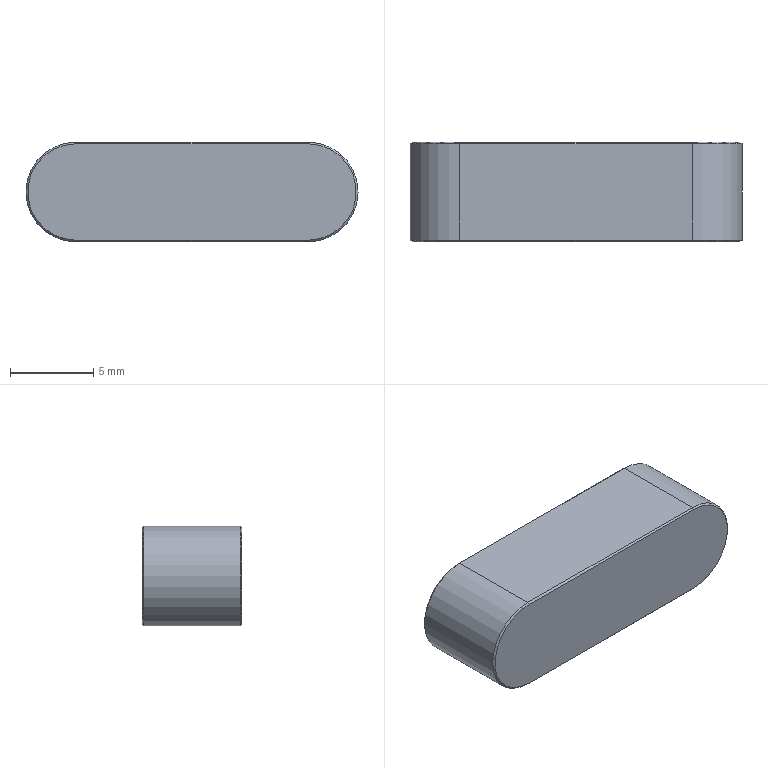Part | STEP file | Type A key 6x6 20L | 1 solid | 14 faces | box 20 x 6 x 6 mm | volume 673.18 mm3 | plane 8 | cone 4 | cylinder 2 | commonest cylinder face diameters 6 x2
STEP:
#1=CARTESIAN_POINT('',(0.,0.,0.));
#2=DIRECTION('',(0.,0.,1.));
#3=DIRECTION('',(1.,0.,0.));
#4=AXIS2_PLACEMENT_3D('',#1,#2,#3);
#5=CARTESIAN_POINT('',(-7.,2.9,-3.));
#6=VERTEX_POINT('',#5);
#7=CARTESIAN_POINT('',(-7.,-2.9,-3.));
#8=VERTEX_POINT('',#7);
#9=CARTESIAN_POINT('',(-7.,3.,-3.));
#10=DIRECTION('',(0.,-1.,0.));
#11=VECTOR('',#10,1.);
#12=LINE('',#9,#11);
#13=CARTESIAN_POINT('',(-7.,3.,0.));
#14=DIRECTION('',(0.,-1.,0.));
#15=DIRECTION('',(0.,0.,-1.));
#16=AXIS2_PLACEMENT_3D('',#13,#14,#15);
#17=CYLINDRICAL_SURFACE('',#16,3.);
#18=CARTESIAN_POINT('',(6.283,0.));
#19=DIRECTION('',(0.,1.));
#20=VECTOR('',#19,1.);
#21=LINE('',#18,#20);
#22=(GEOMETRIC_REPRESENTATION_CONTEXT(2)PARAMETRIC_REPRESENTATION_CONTEXT()REPRESENTATION_CONTEXT('',''));
#23=DEFINITIONAL_REPRESENTATION('',(#21),#22);
#24=PCURVE('',#17,#23);
#25=CARTESIAN_POINT('',(-7.,3.,-3.));
#26=DIRECTION('',(0.,0.,1.));
#27=DIRECTION('',(1.,0.,0.));
#28=AXIS2_PLACEMENT_3D('',#25,#26,#27);
#29=PLANE('',#28);
#30=CARTESIAN_POINT('',(0.,0.));
#31=DIRECTION('',(0.,-1.));
#32=VECTOR('',#31,1.);
#33=LINE('',#30,#32);
#34=(GEOMETRIC_REPRESENTATION_CONTEXT(2)PARAMETRIC_REPRESENTATION_CONTEXT()REPRESENTATION_CONTEXT('',''));
#35=DEFINITIONAL_REPRESENTATION('',(#33),#34);
#36=PCURVE('',#29,#35);
#37=SURFACE_CURVE('',#12,(#24,#36),.PCURVE_S1.);
#38=EDGE_CURVE('',#6,#8,#37,.T.);
#39=ORIENTED_EDGE('',*,*,#38,.T.);
#40=CARTESIAN_POINT('',(-7.,-2.9,3.));
#41=VERTEX_POINT('',#40);
#42=CARTESIAN_POINT('',(-7.,-2.9,0.));
#43=DIRECTION('',(0.,1.,0.));
#44=DIRECTION('',(0.,0.,1.));
#45=AXIS2_PLACEMENT_3D('',#42,#43,#44);
#46=CIRCLE('',#45,3.);
#47=CARTESIAN_POINT('',(9.425,5.9));
#48=DIRECTION('',(-1.,0.));
#49=VECTOR('',#48,1.);
#50=LINE('',#47,#49);
#51=(GEOMETRIC_REPRESENTATION_CONTEXT(2)PARAMETRIC_REPRESENTATION_CONTEXT()REPRESENTATION_CONTEXT('',''));
#52=DEFINITIONAL_REPRESENTATION('',(#50),#51);
#53=PCURVE('',#17,#52);
#54=CARTESIAN_POINT('',(-7.,-2.9,0.));
#55=DIRECTION('',(0.,1.,0.));
#56=DIRECTION('',(0.,0.,1.));
#57=AXIS2_PLACEMENT_3D('',#54,#55,#56);
#58=CONICAL_SURFACE('',#57,3.,0.7854);
#59=CARTESIAN_POINT('',(0.,0.));
#60=DIRECTION('',(1.,0.));
#61=VECTOR('',#60,1.);
#62=LINE('',#59,#61);
#63=(GEOMETRIC_REPRESENTATION_CONTEXT(2)PARAMETRIC_REPRESENTATION_CONTEXT()REPRESENTATION_CONTEXT('',''));
#64=DEFINITIONAL_REPRESENTATION('',(#62),#63);
#65=PCURVE('',#58,#64);
#66=SURFACE_CURVE('',#46,(#53,#65),.PCURVE_S1.);
#67=EDGE_CURVE('',#8,#41,#66,.T.);
#68=ORIENTED_EDGE('',*,*,#67,.T.);
#69=CARTESIAN_POINT('',(-7.,2.9,3.));
#70=VERTEX_POINT('',#69);
#71=CARTESIAN_POINT('',(-7.,3.,3.));
#72=DIRECTION('',(0.,-1.,0.));
#73=VECTOR('',#72,1.);
#74=LINE('',#71,#73);
#75=CARTESIAN_POINT('',(3.142,0.));
#76=DIRECTION('',(0.,1.));
#77=VECTOR('',#76,1.);
#78=LINE('',#75,#77);
#79=(GEOMETRIC_REPRESENTATION_CONTEXT(2)PARAMETRIC_REPRESENTATION_CONTEXT()REPRESENTATION_CONTEXT('',''));
#80=DEFINITIONAL_REPRESENTATION('',(#78),#79);
#81=PCURVE('',#17,#80);
#82=CARTESIAN_POINT('',(-7.,3.,3.));
#83=DIRECTION('',(0.,0.,-1.));
#84=DIRECTION('',(-1.,0.,0.));
#85=AXIS2_PLACEMENT_3D('',#82,#83,#84);
#86=PLANE('',#85);
#87=CARTESIAN_POINT('',(0.,0.));
#88=DIRECTION('',(0.,-1.));
#89=VECTOR('',#88,1.);
#90=LINE('',#87,#89);
#91=(GEOMETRIC_REPRESENTATION_CONTEXT(2)PARAMETRIC_REPRESENTATION_CONTEXT()REPRESENTATION_CONTEXT('',''));
#92=DEFINITIONAL_REPRESENTATION('',(#90),#91);
#93=PCURVE('',#86,#92);
#94=SURFACE_CURVE('',#74,(#81,#93),.PCURVE_S1.);
#95=EDGE_CURVE('',#70,#41,#94,.T.);
#96=ORIENTED_EDGE('',*,*,#95,.F.);
#97=CARTESIAN_POINT('',(-7.,2.9,0.));
#98=DIRECTION('',(0.,-1.,0.));
#99=DIRECTION('',(0.,0.,1.));
#100=AXIS2_PLACEMENT_3D('',#97,#98,#99);
#101=CIRCLE('',#100,3.);
#102=CARTESIAN_POINT('',(3.142,0.1));
#103=DIRECTION('',(1.,0.));
#104=VECTOR('',#103,1.);
#105=LINE('',#102,#104);
#106=(GEOMETRIC_REPRESENTATION_CONTEXT(2)PARAMETRIC_REPRESENTATION_CONTEXT()REPRESENTATION_CONTEXT('',''));
#107=DEFINITIONAL_REPRESENTATION('',(#105),#106);
#108=PCURVE('',#17,#107);
#109=CARTESIAN_POINT('',(-7.,3.,0.));
#110=DIRECTION('',(0.,-1.,0.));
#111=DIRECTION('',(0.,0.,-1.));
#112=AXIS2_PLACEMENT_3D('',#109,#110,#111);
#113=CONICAL_SURFACE('',#112,2.9,0.7854);
#114=CARTESIAN_POINT('',(3.142,0.1));
#115=DIRECTION('',(1.,0.));
#116=VECTOR('',#115,1.);
#117=LINE('',#114,#116);
#118=(GEOMETRIC_REPRESENTATION_CONTEXT(2)PARAMETRIC_REPRESENTATION_CONTEXT()REPRESENTATION_CONTEXT('',''));
#119=DEFINITIONAL_REPRESENTATION('',(#117),#118);
#120=PCURVE('',#113,#119);
#121=SURFACE_CURVE('',#101,(#108,#120),.PCURVE_S1.);
#122=EDGE_CURVE('',#70,#6,#121,.T.);
#123=ORIENTED_EDGE('',*,*,#122,.T.);
#124=EDGE_LOOP('',(#39,#68,#96,#123));
#125=FACE_BOUND('',#124,.T.);
#126=ADVANCED_FACE('',(#125),#17,.T.);
#127=ORIENTED_EDGE('',*,*,#95,.T.);
#128=CARTESIAN_POINT('',(7.,-2.9,3.));
#129=VERTEX_POINT('',#128);
#130=CARTESIAN_POINT('',(-7.,-2.9,3.));
#131=DIRECTION('',(1.,0.,0.));
#132=VECTOR('',#131,1.);
#133=LINE('',#130,#132);
#134=CARTESIAN_POINT('',(0.,-5.9));
#135=DIRECTION('',(-1.,0.));
#136=VECTOR('',#135,1.);
#137=LINE('',#134,#136);
#138=(GEOMETRIC_REPRESENTATION_CONTEXT(2)PARAMETRIC_REPRESENTATION_CONTEXT()REPRESENTATION_CONTEXT('',''));
#139=DEFINITIONAL_REPRESENTATION('',(#137),#138);
#140=PCURVE('',#86,#139);
#141=CARTESIAN_POINT('',(-7.,-2.9,3.));
#142=DIRECTION('',(0.,0.7071,-0.7071));
#143=DIRECTION('',(1.,0.,0.));
#144=AXIS2_PLACEMENT_3D('',#141,#142,#143);
#145=PLANE('',#144);
#146=CARTESIAN_POINT('',(0.,0.));
#147=DIRECTION('',(1.,0.));
#148=VECTOR('',#147,1.);
#149=LINE('',#146,#148);
#150=(GEOMETRIC_REPRESENTATION_CONTEXT(2)PARAMETRIC_REPRESENTATION_CONTEXT()REPRESENTATION_CONTEXT('',''));
#151=DEFINITIONAL_REPRESENTATION('',(#149),#150);
#152=PCURVE('',#145,#151);
#153=SURFACE_CURVE('',#133,(#140,#152),.PCURVE_S1.);
#154=EDGE_CURVE('',#41,#129,#153,.T.);
#155=ORIENTED_EDGE('',*,*,#154,.T.);
#156=CARTESIAN_POINT('',(7.,2.9,3.));
#157=VERTEX_POINT('',#156);
#158=CARTESIAN_POINT('',(7.,3.,3.));
#159=DIRECTION('',(0.,-1.,0.));
#160=VECTOR('',#159,1.);
#161=LINE('',#158,#160);
#162=CARTESIAN_POINT('',(-14.,0.));
#163=DIRECTION('',(0.,-1.));
#164=VECTOR('',#163,1.);
#165=LINE('',#162,#164);
#166=(GEOMETRIC_REPRESENTATION_CONTEXT(2)PARAMETRIC_REPRESENTATION_CONTEXT()REPRESENTATION_CONTEXT('',''));
#167=DEFINITIONAL_REPRESENTATION('',(#165),#166);
#168=PCURVE('',#86,#167);
#169=CARTESIAN_POINT('',(7.,3.,0.));
#170=DIRECTION('',(0.,-1.,0.));
#171=DIRECTION('',(0.,0.,-1.));
#172=AXIS2_PLACEMENT_3D('',#169,#170,#171);
#173=CYLINDRICAL_SURFACE('',#172,3.);
#174=CARTESIAN_POINT('',(3.142,0.));
#175=DIRECTION('',(0.,1.));
#176=VECTOR('',#175,1.);
#177=LINE('',#174,#176);
#178=(GEOMETRIC_REPRESENTATION_CONTEXT(2)PARAMETRIC_REPRESENTATION_CONTEXT()REPRESENTATION_CONTEXT('',''));
#179=DEFINITIONAL_REPRESENTATION('',(#177),#178);
#180=PCURVE('',#173,#179);
#181=SURFACE_CURVE('',#161,(#168,#180),.PCURVE_S1.);
#182=EDGE_CURVE('',#157,#129,#181,.T.);
#183=ORIENTED_EDGE('',*,*,#182,.F.);
#184=CARTESIAN_POINT('',(-7.,2.9,3.));
#185=DIRECTION('',(-1.,0.,0.));
#186=VECTOR('',#185,1.);
#187=LINE('',#184,#186);
#188=CARTESIAN_POINT('',(0.,-0.1));
#189=DIRECTION('',(1.,0.));
#190=VECTOR('',#189,1.);
#191=LINE('',#188,#190);
#192=(GEOMETRIC_REPRESENTATION_CONTEXT(2)PARAMETRIC_REPRESENTATION_CONTEXT()REPRESENTATION_CONTEXT('',''));
#193=DEFINITIONAL_REPRESENTATION('',(#191),#192);
#194=PCURVE('',#86,#193);
#195=CARTESIAN_POINT('',(-7.,3.,2.9));
#196=DIRECTION('',(0.,0.7071,0.7071));
#197=DIRECTION('',(-1.,0.,0.));
#198=AXIS2_PLACEMENT_3D('',#195,#196,#197);
#199=PLANE('',#198);
#200=CARTESIAN_POINT('',(0.,0.1414));
#201=DIRECTION('',(1.,0.));
#202=VECTOR('',#201,1.);
#203=LINE('',#200,#202);
#204=(GEOMETRIC_REPRESENTATION_CONTEXT(2)PARAMETRIC_REPRESENTATION_CONTEXT()REPRESENTATION_CONTEXT('',''));
#205=DEFINITIONAL_REPRESENTATION('',(#203),#204);
#206=PCURVE('',#199,#205);
#207=SURFACE_CURVE('',#187,(#194,#206),.PCURVE_S1.);
#208=EDGE_CURVE('',#157,#70,#207,.T.);
#209=ORIENTED_EDGE('',*,*,#208,.T.);
#210=EDGE_LOOP('',(#127,#155,#183,#209));
#211=FACE_BOUND('',#210,.T.);
#212=ADVANCED_FACE('',(#211),#86,.F.);
#213=ORIENTED_EDGE('',*,*,#182,.T.);
#214=CARTESIAN_POINT('',(7.,-2.9,-3.));
#215=VERTEX_POINT('',#214);
#216=CARTESIAN_POINT('',(7.,-2.9,0.));
#217=DIRECTION('',(0.,1.,0.));
#218=DIRECTION('',(0.,0.,1.));
#219=AXIS2_PLACEMENT_3D('',#216,#217,#218);
#220=CIRCLE('',#219,3.);
#221=CARTESIAN_POINT('',(3.142,5.9));
#222=DIRECTION('',(-1.,0.));
#223=VECTOR('',#222,1.);
#224=LINE('',#221,#223);
#225=(GEOMETRIC_REPRESENTATION_CONTEXT(2)PARAMETRIC_REPRESENTATION_CONTEXT()REPRESENTATION_CONTEXT('',''));
#226=DEFINITIONAL_REPRESENTATION('',(#224),#225);
#227=PCURVE('',#173,#226);
#228=CARTESIAN_POINT('',(7.,-2.9,0.));
#229=DIRECTION('',(0.,1.,0.));
#230=DIRECTION('',(0.,0.,1.));
#231=AXIS2_PLACEMENT_3D('',#228,#229,#230);
#232=CONICAL_SURFACE('',#231,3.,0.7854);
#233=CARTESIAN_POINT('',(0.,0.));
#234=DIRECTION('',(1.,0.));
#235=VECTOR('',#234,1.);
#236=LINE('',#233,#235);
#237=(GEOMETRIC_REPRESENTATION_CONTEXT(2)PARAMETRIC_REPRESENTATION_CONTEXT()REPRESENTATION_CONTEXT('',''));
#238=DEFINITIONAL_REPRESENTATION('',(#236),#237);
#239=PCURVE('',#232,#238);
#240=SURFACE_CURVE('',#220,(#227,#239),.PCURVE_S1.);
#241=EDGE_CURVE('',#129,#215,#240,.T.);
#242=ORIENTED_EDGE('',*,*,#241,.T.);
#243=CARTESIAN_POINT('',(7.,2.9,-3.));
#244=VERTEX_POINT('',#243);
#245=CARTESIAN_POINT('',(7.,3.,-3.));
#246=DIRECTION('',(0.,-1.,0.));
#247=VECTOR('',#246,1.);
#248=LINE('',#245,#247);
#249=CARTESIAN_POINT('',(0.,0.));
#250=DIRECTION('',(0.,1.));
#251=VECTOR('',#250,1.);
#252=LINE('',#249,#251);
#253=(GEOMETRIC_REPRESENTATION_CONTEXT(2)PARAMETRIC_REPRESENTATION_CONTEXT()REPRESENTATION_CONTEXT('',''));
#254=DEFINITIONAL_REPRESENTATION('',(#252),#253);
#255=PCURVE('',#173,#254);
#256=CARTESIAN_POINT('',(14.,0.));
#257=DIRECTION('',(0.,-1.));
#258=VECTOR('',#257,1.);
#259=LINE('',#256,#258);
#260=(GEOMETRIC_REPRESENTATION_CONTEXT(2)PARAMETRIC_REPRESENTATION_CONTEXT()REPRESENTATION_CONTEXT('',''));
#261=DEFINITIONAL_REPRESENTATION('',(#259),#260);
#262=PCURVE('',#29,#261);
#263=SURFACE_CURVE('',#248,(#255,#262),.PCURVE_S1.);
#264=EDGE_CURVE('',#244,#215,#263,.T.);
#265=ORIENTED_EDGE('',*,*,#264,.F.);
#266=CARTESIAN_POINT('',(7.,2.9,0.));
#267=DIRECTION('',(0.,-1.,0.));
#268=DIRECTION('',(0.,0.,1.));
#269=AXIS2_PLACEMENT_3D('',#266,#267,#268);
#270=CIRCLE('',#269,3.);
#271=CARTESIAN_POINT('',(-3.142,0.1));
#272=DIRECTION('',(1.,0.));
#273=VECTOR('',#272,1.);
#274=LINE('',#271,#273);
#275=(GEOMETRIC_REPRESENTATION_CONTEXT(2)PARAMETRIC_REPRESENTATION_CONTEXT()REPRESENTATION_CONTEXT('',''));
#276=DEFINITIONAL_REPRESENTATION('',(#274),#275);
#277=PCURVE('',#173,#276);
#278=CARTESIAN_POINT('',(7.,3.,0.));
#279=DIRECTION('',(0.,-1.,0.));
#280=DIRECTION('',(0.,0.,-1.));
#281=AXIS2_PLACEMENT_3D('',#278,#279,#280);
#282=CONICAL_SURFACE('',#281,2.9,0.7854);
#283=CARTESIAN_POINT('',(-3.142,0.1));
#284=DIRECTION('',(1.,0.));
#285=VECTOR('',#284,1.);
#286=LINE('',#283,#285);
#287=(GEOMETRIC_REPRESENTATION_CONTEXT(2)PARAMETRIC_REPRESENTATION_CONTEXT()REPRESENTATION_CONTEXT('',''));
#288=DEFINITIONAL_REPRESENTATION('',(#286),#287);
#289=PCURVE('',#282,#288);
#290=SURFACE_CURVE('',#270,(#277,#289),.PCURVE_S1.);
#291=EDGE_CURVE('',#244,#157,#290,.T.);
#292=ORIENTED_EDGE('',*,*,#291,.T.);
#293=EDGE_LOOP('',(#213,#242,#265,#292));
#294=FACE_BOUND('',#293,.T.);
#295=ADVANCED_FACE('',(#294),#173,.T.);
#296=ORIENTED_EDGE('',*,*,#264,.T.);
#297=CARTESIAN_POINT('',(-7.,-2.9,-3.));
#298=DIRECTION('',(-1.,0.,0.));
#299=VECTOR('',#298,1.);
#300=LINE('',#297,#299);
#301=CARTESIAN_POINT('',(0.,-5.9));
#302=DIRECTION('',(-1.,0.));
#303=VECTOR('',#302,1.);
#304=LINE('',#301,#303);
#305=(GEOMETRIC_REPRESENTATION_CONTEXT(2)PARAMETRIC_REPRESENTATION_CONTEXT()REPRESENTATION_CONTEXT('',''));
#306=DEFINITIONAL_REPRESENTATION('',(#304),#305);
#307=PCURVE('',#29,#306);
#308=CARTESIAN_POINT('',(-7.,-2.9,-3.));
#309=DIRECTION('',(0.,0.7071,0.7071));
#310=DIRECTION('',(-1.,0.,0.));
#311=AXIS2_PLACEMENT_3D('',#308,#309,#310);
#312=PLANE('',#311);
#313=CARTESIAN_POINT('',(0.,0.));
#314=DIRECTION('',(1.,0.));
#315=VECTOR('',#314,1.);
#316=LINE('',#313,#315);
#317=(GEOMETRIC_REPRESENTATION_CONTEXT(2)PARAMETRIC_REPRESENTATION_CONTEXT()REPRESENTATION_CONTEXT('',''));
#318=DEFINITIONAL_REPRESENTATION('',(#316),#317);
#319=PCURVE('',#312,#318);
#320=SURFACE_CURVE('',#300,(#307,#319),.PCURVE_S1.);
#321=EDGE_CURVE('',#215,#8,#320,.T.);
#322=ORIENTED_EDGE('',*,*,#321,.T.);
#323=ORIENTED_EDGE('',*,*,#38,.F.);
#324=CARTESIAN_POINT('',(7.,2.9,-3.));
#325=DIRECTION('',(1.,0.,0.));
#326=VECTOR('',#325,1.);
#327=LINE('',#324,#326);
#328=CARTESIAN_POINT('',(14.,-0.1));
#329=DIRECTION('',(1.,0.));
#330=VECTOR('',#329,1.);
#331=LINE('',#328,#330);
#332=(GEOMETRIC_REPRESENTATION_CONTEXT(2)PARAMETRIC_REPRESENTATION_CONTEXT()REPRESENTATION_CONTEXT('',''));
#333=DEFINITIONAL_REPRESENTATION('',(#331),#332);
#334=PCURVE('',#29,#333);
#335=CARTESIAN_POINT('',(-7.,3.,-2.9));
#336=DIRECTION('',(0.,0.7071,-0.7071));
#337=DIRECTION('',(1.,0.,0.));
#338=AXIS2_PLACEMENT_3D('',#335,#336,#337);
#339=PLANE('',#338);
#340=CARTESIAN_POINT('',(14.,0.1414));
#341=DIRECTION('',(1.,0.));
#342=VECTOR('',#341,1.);
#343=LINE('',#340,#342);
#344=(GEOMETRIC_REPRESENTATION_CONTEXT(2)PARAMETRIC_REPRESENTATION_CONTEXT()REPRESENTATION_CONTEXT('',''));
#345=DEFINITIONAL_REPRESENTATION('',(#343),#344);
#346=PCURVE('',#339,#345);
#347=SURFACE_CURVE('',#327,(#334,#346),.PCURVE_S1.);
#348=EDGE_CURVE('',#6,#244,#347,.T.);
#349=ORIENTED_EDGE('',*,*,#348,.T.);
#350=EDGE_LOOP('',(#296,#322,#323,#349));
#351=FACE_BOUND('',#350,.T.);
#352=ADVANCED_FACE('',(#351),#29,.F.);
#353=CARTESIAN_POINT('',(-7.,3.,-2.9));
#354=VERTEX_POINT('',#353);
#355=CARTESIAN_POINT('',(-7.,3.,2.9));
#356=VERTEX_POINT('',#355);
#357=CARTESIAN_POINT('',(-7.,3.,0.));
#358=DIRECTION('',(0.,1.,0.));
#359=DIRECTION('',(0.,0.,1.));
#360=AXIS2_PLACEMENT_3D('',#357,#358,#359);
#361=CIRCLE('',#360,2.9);
#362=CARTESIAN_POINT('',(-7.,3.,0.));
#363=DIRECTION('',(0.,1.,0.));
#364=DIRECTION('',(0.,0.,1.));
#365=AXIS2_PLACEMENT_3D('',#362,#363,#364);
#366=PLANE('',#365);
#367=CARTESIAN_POINT('',(0.,0.));
#368=DIRECTION('',(1.,0.));
#369=AXIS2_PLACEMENT_2D('',#367,#368);
#370=CIRCLE('',#369,2.9);
#371=(GEOMETRIC_REPRESENTATION_CONTEXT(2)PARAMETRIC_REPRESENTATION_CONTEXT()REPRESENTATION_CONTEXT('',''));
#372=DEFINITIONAL_REPRESENTATION('',(#370),#371);
#373=PCURVE('',#366,#372);
#374=CARTESIAN_POINT('',(9.425,0.));
#375=DIRECTION('',(-1.,0.));
#376=VECTOR('',#375,1.);
#377=LINE('',#374,#376);
#378=(GEOMETRIC_REPRESENTATION_CONTEXT(2)PARAMETRIC_REPRESENTATION_CONTEXT()REPRESENTATION_CONTEXT('',''));
#379=DEFINITIONAL_REPRESENTATION('',(#377),#378);
#380=PCURVE('',#113,#379);
#381=SURFACE_CURVE('',#361,(#373,#380),.PCURVE_S1.);
#382=EDGE_CURVE('',#354,#356,#381,.T.);
#383=ORIENTED_EDGE('',*,*,#382,.T.);
#384=CARTESIAN_POINT('',(7.,3.,2.9));
#385=VERTEX_POINT('',#384);
#386=CARTESIAN_POINT('',(7.,3.,2.9));
#387=DIRECTION('',(1.,0.,0.));
#388=VECTOR('',#387,1.);
#389=LINE('',#386,#388);
#390=CARTESIAN_POINT('',(2.9,14.));
#391=DIRECTION('',(0.,1.));
#392=VECTOR('',#391,1.);
#393=LINE('',#390,#392);
#394=(GEOMETRIC_REPRESENTATION_CONTEXT(2)PARAMETRIC_REPRESENTATION_CONTEXT()REPRESENTATION_CONTEXT('',''));
#395=DEFINITIONAL_REPRESENTATION('',(#393),#394);
#396=PCURVE('',#366,#395);
#397=CARTESIAN_POINT('',(-14.,0.));
#398=DIRECTION('',(-1.,0.));
#399=VECTOR('',#398,1.);
#400=LINE('',#397,#399);
#401=(GEOMETRIC_REPRESENTATION_CONTEXT(2)PARAMETRIC_REPRESENTATION_CONTEXT()REPRESENTATION_CONTEXT('',''));
#402=DEFINITIONAL_REPRESENTATION('',(#400),#401);
#403=PCURVE('',#199,#402);
#404=SURFACE_CURVE('',#389,(#396,#403),.PCURVE_S1.);
#405=EDGE_CURVE('',#356,#385,#404,.T.);
#406=ORIENTED_EDGE('',*,*,#405,.T.);
#407=CARTESIAN_POINT('',(7.,3.,-2.9));
#408=VERTEX_POINT('',#407);
#409=CARTESIAN_POINT('',(7.,3.,0.));
#410=DIRECTION('',(0.,1.,0.));
#411=DIRECTION('',(0.,0.,1.));
#412=AXIS2_PLACEMENT_3D('',#409,#410,#411);
#413=CIRCLE('',#412,2.9);
#414=CARTESIAN_POINT('',(0.,14.));
#415=DIRECTION('',(1.,0.));
#416=AXIS2_PLACEMENT_2D('',#414,#415);
#417=CIRCLE('',#416,2.9);
#418=(GEOMETRIC_REPRESENTATION_CONTEXT(2)PARAMETRIC_REPRESENTATION_CONTEXT()REPRESENTATION_CONTEXT('',''));
#419=DEFINITIONAL_REPRESENTATION('',(#417),#418);
#420=PCURVE('',#366,#419);
#421=CARTESIAN_POINT('',(3.142,0.));
#422=DIRECTION('',(-1.,0.));
#423=VECTOR('',#422,1.);
#424=LINE('',#421,#423);
#425=(GEOMETRIC_REPRESENTATION_CONTEXT(2)PARAMETRIC_REPRESENTATION_CONTEXT()REPRESENTATION_CONTEXT('',''));
#426=DEFINITIONAL_REPRESENTATION('',(#424),#425);
#427=PCURVE('',#282,#426);
#428=SURFACE_CURVE('',#413,(#420,#427),.PCURVE_S1.);
#429=EDGE_CURVE('',#385,#408,#428,.T.);
#430=ORIENTED_EDGE('',*,*,#429,.T.);
#431=CARTESIAN_POINT('',(-7.,3.,-2.9));
#432=DIRECTION('',(-1.,0.,0.));
#433=VECTOR('',#432,1.);
#434=LINE('',#431,#433);
#435=CARTESIAN_POINT('',(-2.9,0.));
#436=DIRECTION('',(0.,-1.));
#437=VECTOR('',#436,1.);
#438=LINE('',#435,#437);
#439=(GEOMETRIC_REPRESENTATION_CONTEXT(2)PARAMETRIC_REPRESENTATION_CONTEXT()REPRESENTATION_CONTEXT('',''));
#440=DEFINITIONAL_REPRESENTATION('',(#438),#439);
#441=PCURVE('',#366,#440);
#442=CARTESIAN_POINT('',(0.,0.));
#443=DIRECTION('',(-1.,0.));
#444=VECTOR('',#443,1.);
#445=LINE('',#442,#444);
#446=(GEOMETRIC_REPRESENTATION_CONTEXT(2)PARAMETRIC_REPRESENTATION_CONTEXT()REPRESENTATION_CONTEXT('',''));
#447=DEFINITIONAL_REPRESENTATION('',(#445),#446);
#448=PCURVE('',#339,#447);
#449=SURFACE_CURVE('',#434,(#441,#448),.PCURVE_S1.);
#450=EDGE_CURVE('',#408,#354,#449,.T.);
#451=ORIENTED_EDGE('',*,*,#450,.T.);
#452=EDGE_LOOP('',(#383,#406,#430,#451));
#453=FACE_BOUND('',#452,.T.);
#454=ADVANCED_FACE('',(#453),#366,.T.);
#455=CARTESIAN_POINT('',(7.,-3.,-2.9));
#456=VERTEX_POINT('',#455);
#457=CARTESIAN_POINT('',(7.,-3.,2.9));
#458=VERTEX_POINT('',#457);
#459=CARTESIAN_POINT('',(7.,-3.,0.));
#460=DIRECTION('',(0.,-1.,0.));
#461=DIRECTION('',(0.,0.,1.));
#462=AXIS2_PLACEMENT_3D('',#459,#460,#461);
#463=CIRCLE('',#462,2.9);
#464=CARTESIAN_POINT('',(-7.,-3.,0.));
#465=DIRECTION('',(0.,1.,0.));
#466=DIRECTION('',(0.,0.,1.));
#467=AXIS2_PLACEMENT_3D('',#464,#465,#466);
#468=PLANE('',#467);
#469=CARTESIAN_POINT('',(2.9,14.));
#470=CARTESIAN_POINT('',(2.9,8.977));
#471=CARTESIAN_POINT('',(-1.45,11.489));
#472=CARTESIAN_POINT('',(-5.8,14.));
#473=CARTESIAN_POINT('',(-1.45,16.511));
#474=CARTESIAN_POINT('',(2.9,19.023));
#475=CARTESIAN_POINT('',(2.9,14.));
#476=(BOUNDED_CURVE()B_SPLINE_CURVE(2,(#469,#470,#471,#472,#473,#474,#475),.UNSPECIFIED.,.T.,.F.)B_SPLINE_CURVE_WITH_KNOTS((1,2,2,2,2,1),(-2.094,0.,2.094,4.189,6.283,8.378),.UNSPECIFIED.)CURVE()GEOMETRIC_REPRESENTATION_ITEM()RATIONAL_B_SPLINE_CURVE((1.,0.5,1.,0.5,1.,0.5,1.))REPRESENTATION_ITEM(''));
#477=(GEOMETRIC_REPRESENTATION_CONTEXT(2)PARAMETRIC_REPRESENTATION_CONTEXT()REPRESENTATION_CONTEXT('',''));
#478=DEFINITIONAL_REPRESENTATION('',(#476),#477);
#479=PCURVE('',#468,#478);
#480=CARTESIAN_POINT('',(6.283,-0.1));
#481=DIRECTION('',(-1.,0.));
#482=VECTOR('',#481,1.);
#483=LINE('',#480,#482);
#484=(GEOMETRIC_REPRESENTATION_CONTEXT(2)PARAMETRIC_REPRESENTATION_CONTEXT()REPRESENTATION_CONTEXT('',''));
#485=DEFINITIONAL_REPRESENTATION('',(#483),#484);
#486=PCURVE('',#232,#485);
#487=SURFACE_CURVE('',#463,(#479,#486),.PCURVE_S1.);
#488=EDGE_CURVE('',#456,#458,#487,.T.);
#489=ORIENTED_EDGE('',*,*,#488,.T.);
#490=CARTESIAN_POINT('',(-7.,-3.,2.9));
#491=VERTEX_POINT('',#490);
#492=CARTESIAN_POINT('',(-7.,-3.,2.9));
#493=DIRECTION('',(-1.,0.,0.));
#494=VECTOR('',#493,1.);
#495=LINE('',#492,#494);
#496=CARTESIAN_POINT('',(2.9,0.));
#497=DIRECTION('',(0.,-1.));
#498=VECTOR('',#497,1.);
#499=LINE('',#496,#498);
#500=(GEOMETRIC_REPRESENTATION_CONTEXT(2)PARAMETRIC_REPRESENTATION_CONTEXT()REPRESENTATION_CONTEXT('',''));
#501=DEFINITIONAL_REPRESENTATION('',(#499),#500);
#502=PCURVE('',#468,#501);
#503=CARTESIAN_POINT('',(0.,0.1414));
#504=DIRECTION('',(-1.,0.));
#505=VECTOR('',#504,1.);
#506=LINE('',#503,#505);
#507=(GEOMETRIC_REPRESENTATION_CONTEXT(2)PARAMETRIC_REPRESENTATION_CONTEXT()REPRESENTATION_CONTEXT('',''));
#508=DEFINITIONAL_REPRESENTATION('',(#506),#507);
#509=PCURVE('',#145,#508);
#510=SURFACE_CURVE('',#495,(#502,#509),.PCURVE_S1.);
#511=EDGE_CURVE('',#458,#491,#510,.T.);
#512=ORIENTED_EDGE('',*,*,#511,.T.);
#513=CARTESIAN_POINT('',(-7.,-3.,-2.9));
#514=VERTEX_POINT('',#513);
#515=CARTESIAN_POINT('',(-7.,-3.,0.));
#516=DIRECTION('',(0.,-1.,0.));
#517=DIRECTION('',(0.,0.,1.));
#518=AXIS2_PLACEMENT_3D('',#515,#516,#517);
#519=CIRCLE('',#518,2.9);
#520=CARTESIAN_POINT('',(2.9,0.));
#521=CARTESIAN_POINT('',(2.9,-5.023));
#522=CARTESIAN_POINT('',(-1.45,-2.511));
#523=CARTESIAN_POINT('',(-5.8,0.));
#524=CARTESIAN_POINT('',(-1.45,2.511));
#525=CARTESIAN_POINT('',(2.9,5.023));
#526=CARTESIAN_POINT('',(2.9,0.));
#527=(BOUNDED_CURVE()B_SPLINE_CURVE(2,(#520,#521,#522,#523,#524,#525,#526),.UNSPECIFIED.,.T.,.F.)B_SPLINE_CURVE_WITH_KNOTS((1,2,2,2,2,1),(-2.094,0.,2.094,4.189,6.283,8.378),.UNSPECIFIED.)CURVE()GEOMETRIC_REPRESENTATION_ITEM()RATIONAL_B_SPLINE_CURVE((1.,0.5,1.,0.5,1.,0.5,1.))REPRESENTATION_ITEM(''));
#528=(GEOMETRIC_REPRESENTATION_CONTEXT(2)PARAMETRIC_REPRESENTATION_CONTEXT()REPRESENTATION_CONTEXT('',''));
#529=DEFINITIONAL_REPRESENTATION('',(#527),#528);
#530=PCURVE('',#468,#529);
#531=CARTESIAN_POINT('',(6.283,-0.1));
#532=DIRECTION('',(-1.,0.));
#533=VECTOR('',#532,1.);
#534=LINE('',#531,#533);
#535=(GEOMETRIC_REPRESENTATION_CONTEXT(2)PARAMETRIC_REPRESENTATION_CONTEXT()REPRESENTATION_CONTEXT('',''));
#536=DEFINITIONAL_REPRESENTATION('',(#534),#535);
#537=PCURVE('',#58,#536);
#538=SURFACE_CURVE('',#519,(#530,#537),.PCURVE_S1.);
#539=EDGE_CURVE('',#491,#514,#538,.T.);
#540=ORIENTED_EDGE('',*,*,#539,.T.);
#541=CARTESIAN_POINT('',(-7.,-3.,-2.9));
#542=DIRECTION('',(1.,0.,0.));
#543=VECTOR('',#542,1.);
#544=LINE('',#541,#543);
#545=CARTESIAN_POINT('',(-2.9,0.));
#546=DIRECTION('',(0.,1.));
#547=VECTOR('',#546,1.);
#548=LINE('',#545,#547);
#549=(GEOMETRIC_REPRESENTATION_CONTEXT(2)PARAMETRIC_REPRESENTATION_CONTEXT()REPRESENTATION_CONTEXT('',''));
#550=DEFINITIONAL_REPRESENTATION('',(#548),#549);
#551=PCURVE('',#468,#550);
#552=CARTESIAN_POINT('',(0.,0.1414));
#553=DIRECTION('',(-1.,0.));
#554=VECTOR('',#553,1.);
#555=LINE('',#552,#554);
#556=(GEOMETRIC_REPRESENTATION_CONTEXT(2)PARAMETRIC_REPRESENTATION_CONTEXT()REPRESENTATION_CONTEXT('',''));
#557=DEFINITIONAL_REPRESENTATION('',(#555),#556);
#558=PCURVE('',#312,#557);
#559=SURFACE_CURVE('',#544,(#551,#558),.PCURVE_S1.);
#560=EDGE_CURVE('',#514,#456,#559,.T.);
#561=ORIENTED_EDGE('',*,*,#560,.T.);
#562=EDGE_LOOP('',(#489,#512,#540,#561));
#563=FACE_BOUND('',#562,.T.);
#564=ADVANCED_FACE('',(#563),#468,.F.);
#565=CARTESIAN_POINT('',(7.,-3.,-2.9));
#566=DIRECTION('',(0.,0.7071,-0.7071));
#567=VECTOR('',#566,1.);
#568=LINE('',#565,#567);
#569=CARTESIAN_POINT('',(-14.,0.1414));
#570=DIRECTION('',(0.,-1.));
#571=VECTOR('',#570,1.);
#572=LINE('',#569,#571);
#573=(GEOMETRIC_REPRESENTATION_CONTEXT(2)PARAMETRIC_REPRESENTATION_CONTEXT()REPRESENTATION_CONTEXT('',''));
#574=DEFINITIONAL_REPRESENTATION('',(#572),#573);
#575=PCURVE('',#312,#574);
#576=CARTESIAN_POINT('',(3.142,-0.1));
#577=DIRECTION('',(0.,1.));
#578=VECTOR('',#577,1.);
#579=LINE('',#576,#578);
#580=(GEOMETRIC_REPRESENTATION_CONTEXT(2)PARAMETRIC_REPRESENTATION_CONTEXT()REPRESENTATION_CONTEXT('',''));
#581=DEFINITIONAL_REPRESENTATION('',(#579),#580);
#582=PCURVE('',#232,#581);
#583=SURFACE_CURVE('',#568,(#575,#582),.PCURVE_S1.);
#584=EDGE_CURVE('',#456,#215,#583,.T.);
#585=ORIENTED_EDGE('',*,*,#584,.F.);
#586=ORIENTED_EDGE('',*,*,#560,.F.);
#587=CARTESIAN_POINT('',(-7.,-2.9,-3.));
#588=DIRECTION('',(0.,-0.7071,0.7071));
#589=VECTOR('',#588,1.);
#590=LINE('',#587,#589);
#591=CARTESIAN_POINT('',(0.,0.));
#592=DIRECTION('',(0.,1.));
#593=VECTOR('',#592,1.);
#594=LINE('',#591,#593);
#595=(GEOMETRIC_REPRESENTATION_CONTEXT(2)PARAMETRIC_REPRESENTATION_CONTEXT()REPRESENTATION_CONTEXT('',''));
#596=DEFINITIONAL_REPRESENTATION('',(#594),#595);
#597=PCURVE('',#312,#596);
#598=CARTESIAN_POINT('',(3.142,0.));
#599=DIRECTION('',(0.,-1.));
#600=VECTOR('',#599,1.);
#601=LINE('',#598,#600);
#602=(GEOMETRIC_REPRESENTATION_CONTEXT(2)PARAMETRIC_REPRESENTATION_CONTEXT()REPRESENTATION_CONTEXT('',''));
#603=DEFINITIONAL_REPRESENTATION('',(#601),#602);
#604=PCURVE('',#58,#603);
#605=SURFACE_CURVE('',#590,(#597,#604),.PCURVE_S1.);
#606=EDGE_CURVE('',#8,#514,#605,.T.);
#607=ORIENTED_EDGE('',*,*,#606,.F.);
#608=ORIENTED_EDGE('',*,*,#321,.F.);
#609=EDGE_LOOP('',(#585,#586,#607,#608));
#610=FACE_BOUND('',#609,.T.);
#611=ADVANCED_FACE('',(#610),#312,.F.);
#612=ORIENTED_EDGE('',*,*,#606,.T.);
#613=ORIENTED_EDGE('',*,*,#539,.F.);
#614=CARTESIAN_POINT('',(-7.,-2.9,3.));
#615=DIRECTION('',(0.,-0.7071,-0.7071));
#616=VECTOR('',#615,1.);
#617=LINE('',#614,#616);
#618=CARTESIAN_POINT('',(6.283,0.));
#619=DIRECTION('',(0.,-1.));
#620=VECTOR('',#619,1.);
#621=LINE('',#618,#620);
#622=(GEOMETRIC_REPRESENTATION_CONTEXT(2)PARAMETRIC_REPRESENTATION_CONTEXT()REPRESENTATION_CONTEXT('',''));
#623=DEFINITIONAL_REPRESENTATION('',(#621),#622);
#624=PCURVE('',#58,#623);
#625=CARTESIAN_POINT('',(0.,0.));
#626=DIRECTION('',(0.,1.));
#627=VECTOR('',#626,1.);
#628=LINE('',#625,#627);
#629=(GEOMETRIC_REPRESENTATION_CONTEXT(2)PARAMETRIC_REPRESENTATION_CONTEXT()REPRESENTATION_CONTEXT('',''));
#630=DEFINITIONAL_REPRESENTATION('',(#628),#629);
#631=PCURVE('',#145,#630);
#632=SURFACE_CURVE('',#617,(#624,#631),.PCURVE_S1.);
#633=EDGE_CURVE('',#41,#491,#632,.T.);
#634=ORIENTED_EDGE('',*,*,#633,.F.);
#635=ORIENTED_EDGE('',*,*,#67,.F.);
#636=EDGE_LOOP('',(#612,#613,#634,#635));
#637=FACE_BOUND('',#636,.T.);
#638=ADVANCED_FACE('',(#637),#58,.T.);
#639=ORIENTED_EDGE('',*,*,#584,.T.);
#640=ORIENTED_EDGE('',*,*,#241,.F.);
#641=CARTESIAN_POINT('',(7.,-3.,2.9));
#642=DIRECTION('',(0.,0.7071,0.7071));
#643=VECTOR('',#642,1.);
#644=LINE('',#641,#643);
#645=CARTESIAN_POINT('',(0.,-0.1));
#646=DIRECTION('',(0.,1.));
#647=VECTOR('',#646,1.);
#648=LINE('',#645,#647);
#649=(GEOMETRIC_REPRESENTATION_CONTEXT(2)PARAMETRIC_REPRESENTATION_CONTEXT()REPRESENTATION_CONTEXT('',''));
#650=DEFINITIONAL_REPRESENTATION('',(#648),#649);
#651=PCURVE('',#232,#650);
#652=CARTESIAN_POINT('',(14.,0.1414));
#653=DIRECTION('',(0.,-1.));
#654=VECTOR('',#653,1.);
#655=LINE('',#652,#654);
#656=(GEOMETRIC_REPRESENTATION_CONTEXT(2)PARAMETRIC_REPRESENTATION_CONTEXT()REPRESENTATION_CONTEXT('',''));
#657=DEFINITIONAL_REPRESENTATION('',(#655),#656);
#658=PCURVE('',#145,#657);
#659=SURFACE_CURVE('',#644,(#651,#658),.PCURVE_S1.);
#660=EDGE_CURVE('',#458,#129,#659,.T.);
#661=ORIENTED_EDGE('',*,*,#660,.F.);
#662=ORIENTED_EDGE('',*,*,#488,.F.);
#663=EDGE_LOOP('',(#639,#640,#661,#662));
#664=FACE_BOUND('',#663,.T.);
#665=ADVANCED_FACE('',(#664),#232,.T.);
#666=ORIENTED_EDGE('',*,*,#633,.T.);
#667=ORIENTED_EDGE('',*,*,#511,.F.);
#668=ORIENTED_EDGE('',*,*,#660,.T.);
#669=ORIENTED_EDGE('',*,*,#154,.F.);
#670=EDGE_LOOP('',(#666,#667,#668,#669));
#671=FACE_BOUND('',#670,.T.);
#672=ADVANCED_FACE('',(#671),#145,.F.);
#673=CARTESIAN_POINT('',(7.,2.9,-3.));
#674=DIRECTION('',(0.,0.7071,0.7071));
#675=VECTOR('',#674,1.);
#676=LINE('',#673,#675);
#677=CARTESIAN_POINT('',(14.,0.1414));
#678=DIRECTION('',(0.,-1.));
#679=VECTOR('',#678,1.);
#680=LINE('',#677,#679);
#681=(GEOMETRIC_REPRESENTATION_CONTEXT(2)PARAMETRIC_REPRESENTATION_CONTEXT()REPRESENTATION_CONTEXT('',''));
#682=DEFINITIONAL_REPRESENTATION('',(#680),#681);
#683=PCURVE('',#339,#682);
#684=CARTESIAN_POINT('',(0.,0.1));
#685=DIRECTION('',(0.,-1.));
#686=VECTOR('',#685,1.);
#687=LINE('',#684,#686);
#688=(GEOMETRIC_REPRESENTATION_CONTEXT(2)PARAMETRIC_REPRESENTATION_CONTEXT()REPRESENTATION_CONTEXT('',''));
#689=DEFINITIONAL_REPRESENTATION('',(#687),#688);
#690=PCURVE('',#282,#689);
#691=SURFACE_CURVE('',#676,(#683,#690),.PCURVE_S1.);
#692=EDGE_CURVE('',#244,#408,#691,.T.);
#693=ORIENTED_EDGE('',*,*,#692,.F.);
#694=ORIENTED_EDGE('',*,*,#348,.F.);
#695=CARTESIAN_POINT('',(-7.,3.,-2.9));
#696=DIRECTION('',(0.,-0.7071,-0.7071));
#697=VECTOR('',#696,1.);
#698=LINE('',#695,#697);
#699=CARTESIAN_POINT('',(0.,0.));
#700=DIRECTION('',(0.,1.));
#701=VECTOR('',#700,1.);
#702=LINE('',#699,#701);
#703=(GEOMETRIC_REPRESENTATION_CONTEXT(2)PARAMETRIC_REPRESENTATION_CONTEXT()REPRESENTATION_CONTEXT('',''));
#704=DEFINITIONAL_REPRESENTATION('',(#702),#703);
#705=PCURVE('',#339,#704);
#706=CARTESIAN_POINT('',(6.283,0.));
#707=DIRECTION('',(0.,1.));
#708=VECTOR('',#707,1.);
#709=LINE('',#706,#708);
#710=(GEOMETRIC_REPRESENTATION_CONTEXT(2)PARAMETRIC_REPRESENTATION_CONTEXT()REPRESENTATION_CONTEXT('',''));
#711=DEFINITIONAL_REPRESENTATION('',(#709),#710);
#712=PCURVE('',#113,#711);
#713=SURFACE_CURVE('',#698,(#705,#712),.PCURVE_S1.);
#714=EDGE_CURVE('',#354,#6,#713,.T.);
#715=ORIENTED_EDGE('',*,*,#714,.F.);
#716=ORIENTED_EDGE('',*,*,#450,.F.);
#717=EDGE_LOOP('',(#693,#694,#715,#716));
#718=FACE_BOUND('',#717,.T.);
#719=ADVANCED_FACE('',(#718),#339,.T.);
#720=ORIENTED_EDGE('',*,*,#714,.T.);
#721=ORIENTED_EDGE('',*,*,#122,.F.);
#722=CARTESIAN_POINT('',(-7.,3.,2.9));
#723=DIRECTION('',(0.,-0.7071,0.7071));
#724=VECTOR('',#723,1.);
#725=LINE('',#722,#724);
#726=CARTESIAN_POINT('',(3.142,0.));
#727=DIRECTION('',(0.,1.));
#728=VECTOR('',#727,1.);
#729=LINE('',#726,#728);
#730=(GEOMETRIC_REPRESENTATION_CONTEXT(2)PARAMETRIC_REPRESENTATION_CONTEXT()REPRESENTATION_CONTEXT('',''));
#731=DEFINITIONAL_REPRESENTATION('',(#729),#730);
#732=PCURVE('',#113,#731);
#733=CARTESIAN_POINT('',(0.,0.));
#734=DIRECTION('',(0.,1.));
#735=VECTOR('',#734,1.);
#736=LINE('',#733,#735);
#737=(GEOMETRIC_REPRESENTATION_CONTEXT(2)PARAMETRIC_REPRESENTATION_CONTEXT()REPRESENTATION_CONTEXT('',''));
#738=DEFINITIONAL_REPRESENTATION('',(#736),#737);
#739=PCURVE('',#199,#738);
#740=SURFACE_CURVE('',#725,(#732,#739),.PCURVE_S1.);
#741=EDGE_CURVE('',#356,#70,#740,.T.);
#742=ORIENTED_EDGE('',*,*,#741,.F.);
#743=ORIENTED_EDGE('',*,*,#382,.F.);
#744=EDGE_LOOP('',(#720,#721,#742,#743));
#745=FACE_BOUND('',#744,.T.);
#746=ADVANCED_FACE('',(#745),#113,.T.);
#747=ORIENTED_EDGE('',*,*,#692,.T.);
#748=ORIENTED_EDGE('',*,*,#429,.F.);
#749=CARTESIAN_POINT('',(7.,2.9,3.));
#750=DIRECTION('',(0.,0.7071,-0.7071));
#751=VECTOR('',#750,1.);
#752=LINE('',#749,#751);
#753=CARTESIAN_POINT('',(3.142,0.1));
#754=DIRECTION('',(0.,-1.));
#755=VECTOR('',#754,1.);
#756=LINE('',#753,#755);
#757=(GEOMETRIC_REPRESENTATION_CONTEXT(2)PARAMETRIC_REPRESENTATION_CONTEXT()REPRESENTATION_CONTEXT('',''));
#758=DEFINITIONAL_REPRESENTATION('',(#756),#757);
#759=PCURVE('',#282,#758);
#760=CARTESIAN_POINT('',(-14.,0.1414));
#761=DIRECTION('',(0.,-1.));
#762=VECTOR('',#761,1.);
#763=LINE('',#760,#762);
#764=(GEOMETRIC_REPRESENTATION_CONTEXT(2)PARAMETRIC_REPRESENTATION_CONTEXT()REPRESENTATION_CONTEXT('',''));
#765=DEFINITIONAL_REPRESENTATION('',(#763),#764);
#766=PCURVE('',#199,#765);
#767=SURFACE_CURVE('',#752,(#759,#766),.PCURVE_S1.);
#768=EDGE_CURVE('',#157,#385,#767,.T.);
#769=ORIENTED_EDGE('',*,*,#768,.F.);
#770=ORIENTED_EDGE('',*,*,#291,.F.);
#771=EDGE_LOOP('',(#747,#748,#769,#770));
#772=FACE_BOUND('',#771,.T.);
#773=ADVANCED_FACE('',(#772),#282,.T.);
#774=ORIENTED_EDGE('',*,*,#741,.T.);
#775=ORIENTED_EDGE('',*,*,#208,.F.);
#776=ORIENTED_EDGE('',*,*,#768,.T.);
#777=ORIENTED_EDGE('',*,*,#405,.F.);
#778=EDGE_LOOP('',(#774,#775,#776,#777));
#779=FACE_BOUND('',#778,.T.);
#780=ADVANCED_FACE('',(#779),#199,.T.);
#781=CLOSED_SHELL('',(#126,#212,#295,#352,#454,#564,#611,#638,#665,#672,#719,#746,#773,#780));
#782=MANIFOLD_SOLID_BREP('',#781);
#783=(LENGTH_UNIT()NAMED_UNIT(*)SI_UNIT(.MILLI.,.METRE.));
#784=UNCERTAINTY_MEASURE_WITH_UNIT(LENGTH_MEASURE(0.0000001),#783,'','');
#785=(NAMED_UNIT(*)PLANE_ANGLE_UNIT()SI_UNIT($,.RADIAN.));
#786=(NAMED_UNIT(*)SI_UNIT($,.STERADIAN.)SOLID_ANGLE_UNIT());
#787=(GEOMETRIC_REPRESENTATION_CONTEXT(3)GLOBAL_UNCERTAINTY_ASSIGNED_CONTEXT((#784))GLOBAL_UNIT_ASSIGNED_CONTEXT((#783,#785,#786))REPRESENTATION_CONTEXT('',''));
#788=ADVANCED_BREP_SHAPE_REPRESENTATION('',(#4,#782),#787);